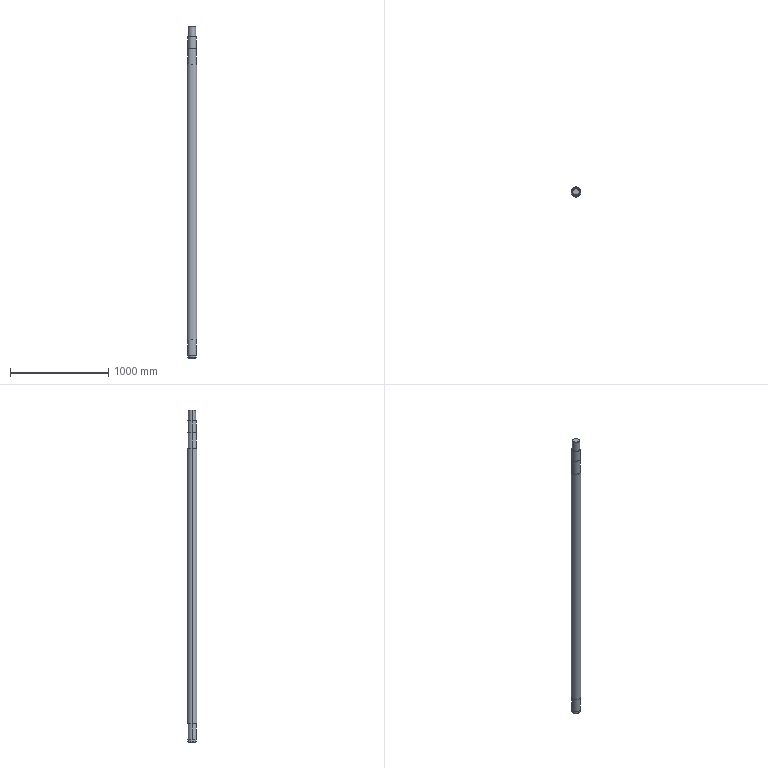Part | SolidWorks | features ICE 7, Chamfer 1, Extrusion 1 | 1 solid | 23 faces | box 100 x 100 x 3375 mm | volume 25329647 mm3 | cylinder 12 | plane 7 | cone 4 | commonest cylinder face diameters 85 x4 90 x4 75 x2 100 x2
STEP:
#1=CARTESIAN_POINT('',(32.5,0.,3610.));
#2=VERTEX_POINT('',#1);
#3=CARTESIAN_POINT('',(-32.5,0.,3610.));
#4=VERTEX_POINT('',#3);
#5=CARTESIAN_POINT('',(0.,0.,3610.));
#6=DIRECTION('',(0.,0.,1.));
#7=DIRECTION('',(1.,0.,0.));
#8=AXIS2_PLACEMENT_3D('',#5,#6,#7);
#9=CIRCLE('',#8,32.5);
#10=EDGE_CURVE('',#2,#4,#9,.T.);
#11=ORIENTED_EDGE('',*,*,#10,.F.);
#12=CARTESIAN_POINT('',(37.5,0.,3605.));
#13=VERTEX_POINT('',#12);
#14=CARTESIAN_POINT('',(32.5,0.,3610.));
#15=DIRECTION('',(0.7071,0.,-0.7071));
#16=VECTOR('',#15,1000.);
#17=LINE('',#14,#16);
#18=EDGE_CURVE('',#2,#13,#17,.T.);
#19=ORIENTED_EDGE('',*,*,#18,.T.);
#20=CARTESIAN_POINT('',(-37.5,0.,3605.));
#21=VERTEX_POINT('',#20);
#22=CARTESIAN_POINT('',(0.,0.,3605.));
#23=DIRECTION('',(0.,0.,-1.));
#24=DIRECTION('',(1.,0.,0.));
#25=AXIS2_PLACEMENT_3D('',#22,#23,#24);
#26=CIRCLE('',#25,37.5);
#27=EDGE_CURVE('',#21,#13,#26,.T.);
#28=ORIENTED_EDGE('',*,*,#27,.F.);
#29=CARTESIAN_POINT('',(-32.5,0.,3610.));
#30=DIRECTION('',(-0.7071,0.,-0.7071));
#31=VECTOR('',#30,1000.);
#32=LINE('',#29,#31);
#33=EDGE_CURVE('',#4,#21,#32,.T.);
#34=ORIENTED_EDGE('',*,*,#33,.F.);
#35=EDGE_LOOP('',(#11,#19,#28,#34));
#36=FACE_OUTER_BOUND('',#35,.T.);
#37=CARTESIAN_POINT('',(0.,0.,3610.));
#38=DIRECTION('',(0.,0.,-1.));
#39=DIRECTION('',(-1.,0.,0.));
#40=AXIS2_PLACEMENT_3D('',#37,#38,#39);
#41=CONICAL_SURFACE('',#40,32.5,0.7854);
#42=ADVANCED_FACE('',(#36),#41,.T.);
#43=CARTESIAN_POINT('',(-37.5,0.,235.));
#44=VERTEX_POINT('',#43);
#45=CARTESIAN_POINT('',(37.5,0.,235.));
#46=VERTEX_POINT('',#45);
#47=CARTESIAN_POINT('',(0.,0.,235.));
#48=DIRECTION('',(0.,0.,-1.));
#49=DIRECTION('',(-1.,0.,0.));
#50=AXIS2_PLACEMENT_3D('',#47,#48,#49);
#51=CIRCLE('',#50,37.5);
#52=EDGE_CURVE('',#44,#46,#51,.T.);
#53=ORIENTED_EDGE('',*,*,#52,.F.);
#54=CARTESIAN_POINT('',(-42.5,0.,240.));
#55=VERTEX_POINT('',#54);
#56=CARTESIAN_POINT('',(-37.5,0.,235.));
#57=DIRECTION('',(-0.7071,0.,0.7071));
#58=VECTOR('',#57,1000.);
#59=LINE('',#56,#58);
#60=EDGE_CURVE('',#44,#55,#59,.T.);
#61=ORIENTED_EDGE('',*,*,#60,.T.);
#62=CARTESIAN_POINT('',(42.5,0.,240.));
#63=VERTEX_POINT('',#62);
#64=CARTESIAN_POINT('',(0.,0.,240.));
#65=DIRECTION('',(0.,0.,1.));
#66=DIRECTION('',(-1.,0.,0.));
#67=AXIS2_PLACEMENT_3D('',#64,#65,#66);
#68=CIRCLE('',#67,42.5);
#69=EDGE_CURVE('',#63,#55,#68,.T.);
#70=ORIENTED_EDGE('',*,*,#69,.F.);
#71=CARTESIAN_POINT('',(37.5,0.,235.));
#72=DIRECTION('',(0.7071,0.,0.7071));
#73=VECTOR('',#72,1000.);
#74=LINE('',#71,#73);
#75=EDGE_CURVE('',#46,#63,#74,.T.);
#76=ORIENTED_EDGE('',*,*,#75,.F.);
#77=EDGE_LOOP('',(#53,#61,#70,#76));
#78=FACE_OUTER_BOUND('',#77,.T.);
#79=CARTESIAN_POINT('',(0.,0.,235.));
#80=DIRECTION('',(0.,0.,1.));
#81=DIRECTION('',(1.,0.,0.));
#82=AXIS2_PLACEMENT_3D('',#79,#80,#81);
#83=CONICAL_SURFACE('',#82,37.5,0.7854);
#84=ADVANCED_FACE('',(#78),#83,.T.);
#85=ORIENTED_EDGE('',*,*,#27,.T.);
#86=CARTESIAN_POINT('',(37.5,0.,3500.));
#87=VERTEX_POINT('',#86);
#88=CARTESIAN_POINT('',(37.5,0.,3610.));
#89=DIRECTION('',(0.,0.,-1.));
#90=VECTOR('',#89,1000.);
#91=LINE('',#88,#90);
#92=EDGE_CURVE('',#13,#87,#91,.T.);
#93=ORIENTED_EDGE('',*,*,#92,.T.);
#94=CARTESIAN_POINT('',(-37.5,0.,3500.));
#95=VERTEX_POINT('',#94);
#96=CARTESIAN_POINT('',(0.,0.,3500.));
#97=DIRECTION('',(0.,0.,1.));
#98=DIRECTION('',(1.,0.,0.));
#99=AXIS2_PLACEMENT_3D('',#96,#97,#98);
#100=CIRCLE('',#99,37.5);
#101=EDGE_CURVE('',#87,#95,#100,.T.);
#102=ORIENTED_EDGE('',*,*,#101,.T.);
#103=CARTESIAN_POINT('',(-37.5,0.,3610.));
#104=DIRECTION('',(0.,0.,-1.));
#105=VECTOR('',#104,1000.);
#106=LINE('',#103,#105);
#107=EDGE_CURVE('',#21,#95,#106,.T.);
#108=ORIENTED_EDGE('',*,*,#107,.F.);
#109=EDGE_LOOP('',(#85,#93,#102,#108));
#110=FACE_OUTER_BOUND('',#109,.T.);
#111=CARTESIAN_POINT('',(0.,0.,3610.));
#112=DIRECTION('',(0.,0.,-1.));
#113=DIRECTION('',(-1.,0.,0.));
#114=AXIS2_PLACEMENT_3D('',#111,#112,#113);
#115=CYLINDRICAL_SURFACE('',#114,37.5);
#116=ADVANCED_FACE('',(#110),#115,.T.);
#117=CARTESIAN_POINT('',(42.5,0.,3500.));
#118=VERTEX_POINT('',#117);
#119=CARTESIAN_POINT('',(-42.5,0.,3500.));
#120=VERTEX_POINT('',#119);
#121=CARTESIAN_POINT('',(0.,0.,3500.));
#122=DIRECTION('',(0.,0.,1.));
#123=DIRECTION('',(1.,0.,0.));
#124=AXIS2_PLACEMENT_3D('',#121,#122,#123);
#125=CIRCLE('',#124,42.5);
#126=EDGE_CURVE('',#118,#120,#125,.T.);
#127=ORIENTED_EDGE('',*,*,#126,.F.);
#128=CARTESIAN_POINT('',(42.5,0.,3380.));
#129=VERTEX_POINT('',#128);
#130=CARTESIAN_POINT('',(42.5,0.,3500.));
#131=DIRECTION('',(0.,0.,-1.));
#132=VECTOR('',#131,1000.);
#133=LINE('',#130,#132);
#134=EDGE_CURVE('',#118,#129,#133,.T.);
#135=ORIENTED_EDGE('',*,*,#134,.T.);
#136=CARTESIAN_POINT('',(-42.5,0.,3380.));
#137=VERTEX_POINT('',#136);
#138=CARTESIAN_POINT('',(0.,0.,3380.));
#139=DIRECTION('',(0.,0.,1.));
#140=DIRECTION('',(1.,0.,0.));
#141=AXIS2_PLACEMENT_3D('',#138,#139,#140);
#142=CIRCLE('',#141,42.5);
#143=EDGE_CURVE('',#129,#137,#142,.T.);
#144=ORIENTED_EDGE('',*,*,#143,.T.);
#145=CARTESIAN_POINT('',(-42.5,0.,3500.));
#146=DIRECTION('',(0.,0.,-1.));
#147=VECTOR('',#146,1000.);
#148=LINE('',#145,#147);
#149=EDGE_CURVE('',#120,#137,#148,.T.);
#150=ORIENTED_EDGE('',*,*,#149,.F.);
#151=EDGE_LOOP('',(#127,#135,#144,#150));
#152=FACE_OUTER_BOUND('',#151,.T.);
#153=CARTESIAN_POINT('',(0.,0.,3500.));
#154=DIRECTION('',(0.,0.,-1.));
#155=DIRECTION('',(-1.,0.,0.));
#156=AXIS2_PLACEMENT_3D('',#153,#154,#155);
#157=CYLINDRICAL_SURFACE('',#156,42.5);
#158=ADVANCED_FACE('',(#152),#157,.T.);
#159=CARTESIAN_POINT('',(45.,0.,3380.));
#160=VERTEX_POINT('',#159);
#161=CARTESIAN_POINT('',(-45.,0.,3380.));
#162=VERTEX_POINT('',#161);
#163=CARTESIAN_POINT('',(0.,0.,3380.));
#164=DIRECTION('',(0.,0.,1.));
#165=DIRECTION('',(1.,0.,0.));
#166=AXIS2_PLACEMENT_3D('',#163,#164,#165);
#167=CIRCLE('',#166,45.);
#168=EDGE_CURVE('',#160,#162,#167,.T.);
#169=ORIENTED_EDGE('',*,*,#168,.F.);
#170=CARTESIAN_POINT('',(45.,0.,3220.));
#171=VERTEX_POINT('',#170);
#172=CARTESIAN_POINT('',(45.,0.,3380.));
#173=DIRECTION('',(0.,0.,-1.));
#174=VECTOR('',#173,1000.);
#175=LINE('',#172,#174);
#176=EDGE_CURVE('',#160,#171,#175,.T.);
#177=ORIENTED_EDGE('',*,*,#176,.T.);
#178=CARTESIAN_POINT('',(-45.,0.,3220.));
#179=VERTEX_POINT('',#178);
#180=CARTESIAN_POINT('',(0.,0.,3220.));
#181=DIRECTION('',(0.,0.,1.));
#182=DIRECTION('',(1.,0.,0.));
#183=AXIS2_PLACEMENT_3D('',#180,#181,#182);
#184=CIRCLE('',#183,45.);
#185=EDGE_CURVE('',#171,#179,#184,.T.);
#186=ORIENTED_EDGE('',*,*,#185,.T.);
#187=CARTESIAN_POINT('',(-45.,0.,3380.));
#188=DIRECTION('',(0.,0.,-1.));
#189=VECTOR('',#188,1000.);
#190=LINE('',#187,#189);
#191=EDGE_CURVE('',#162,#179,#190,.T.);
#192=ORIENTED_EDGE('',*,*,#191,.F.);
#193=EDGE_LOOP('',(#169,#177,#186,#192));
#194=FACE_OUTER_BOUND('',#193,.T.);
#195=CARTESIAN_POINT('',(0.,0.,3380.));
#196=DIRECTION('',(0.,0.,-1.));
#197=DIRECTION('',(-1.,0.,0.));
#198=AXIS2_PLACEMENT_3D('',#195,#196,#197);
#199=CYLINDRICAL_SURFACE('',#198,45.);
#200=ADVANCED_FACE('',(#194),#199,.T.);
#201=CARTESIAN_POINT('',(50.,0.,3220.));
#202=VERTEX_POINT('',#201);
#203=CARTESIAN_POINT('',(-50.,0.,3220.));
#204=VERTEX_POINT('',#203);
#205=CARTESIAN_POINT('',(0.,0.,3220.));
#206=DIRECTION('',(0.,0.,1.));
#207=DIRECTION('',(1.,0.,0.));
#208=AXIS2_PLACEMENT_3D('',#205,#206,#207);
#209=CIRCLE('',#208,50.);
#210=EDGE_CURVE('',#202,#204,#209,.T.);
#211=ORIENTED_EDGE('',*,*,#210,.F.);
#212=CARTESIAN_POINT('',(50.,0.,420.));
#213=VERTEX_POINT('',#212);
#214=CARTESIAN_POINT('',(50.,0.,3220.));
#215=DIRECTION('',(0.,0.,-1.));
#216=VECTOR('',#215,1000.);
#217=LINE('',#214,#216);
#218=EDGE_CURVE('',#202,#213,#217,.T.);
#219=ORIENTED_EDGE('',*,*,#218,.T.);
#220=CARTESIAN_POINT('',(-50.,0.,420.));
#221=VERTEX_POINT('',#220);
#222=CARTESIAN_POINT('',(0.,0.,420.));
#223=DIRECTION('',(0.,0.,1.));
#224=DIRECTION('',(1.,0.,0.));
#225=AXIS2_PLACEMENT_3D('',#222,#223,#224);
#226=CIRCLE('',#225,50.);
#227=EDGE_CURVE('',#213,#221,#226,.T.);
#228=ORIENTED_EDGE('',*,*,#227,.T.);
#229=CARTESIAN_POINT('',(-50.,0.,3220.));
#230=DIRECTION('',(0.,0.,-1.));
#231=VECTOR('',#230,1000.);
#232=LINE('',#229,#231);
#233=EDGE_CURVE('',#204,#221,#232,.T.);
#234=ORIENTED_EDGE('',*,*,#233,.F.);
#235=EDGE_LOOP('',(#211,#219,#228,#234));
#236=FACE_OUTER_BOUND('',#235,.T.);
#237=CARTESIAN_POINT('',(0.,0.,3220.));
#238=DIRECTION('',(0.,0.,-1.));
#239=DIRECTION('',(-1.,0.,0.));
#240=AXIS2_PLACEMENT_3D('',#237,#238,#239);
#241=CYLINDRICAL_SURFACE('',#240,50.);
#242=ADVANCED_FACE('',(#236),#241,.T.);
#243=CARTESIAN_POINT('',(45.,0.,420.));
#244=VERTEX_POINT('',#243);
#245=CARTESIAN_POINT('',(-45.,0.,420.));
#246=VERTEX_POINT('',#245);
#247=CARTESIAN_POINT('',(0.,0.,420.));
#248=DIRECTION('',(0.,0.,1.));
#249=DIRECTION('',(1.,0.,0.));
#250=AXIS2_PLACEMENT_3D('',#247,#248,#249);
#251=CIRCLE('',#250,45.);
#252=EDGE_CURVE('',#244,#246,#251,.T.);
#253=ORIENTED_EDGE('',*,*,#252,.F.);
#254=CARTESIAN_POINT('',(45.,0.,260.));
#255=VERTEX_POINT('',#254);
#256=CARTESIAN_POINT('',(45.,0.,420.));
#257=DIRECTION('',(0.,0.,-1.));
#258=VECTOR('',#257,1000.);
#259=LINE('',#256,#258);
#260=EDGE_CURVE('',#244,#255,#259,.T.);
#261=ORIENTED_EDGE('',*,*,#260,.T.);
#262=CARTESIAN_POINT('',(-45.,0.,260.));
#263=VERTEX_POINT('',#262);
#264=CARTESIAN_POINT('',(0.,0.,260.));
#265=DIRECTION('',(0.,0.,1.));
#266=DIRECTION('',(1.,0.,0.));
#267=AXIS2_PLACEMENT_3D('',#264,#265,#266);
#268=CIRCLE('',#267,45.);
#269=EDGE_CURVE('',#255,#263,#268,.T.);
#270=ORIENTED_EDGE('',*,*,#269,.T.);
#271=CARTESIAN_POINT('',(-45.,0.,420.));
#272=DIRECTION('',(0.,0.,-1.));
#273=VECTOR('',#272,1000.);
#274=LINE('',#271,#273);
#275=EDGE_CURVE('',#246,#263,#274,.T.);
#276=ORIENTED_EDGE('',*,*,#275,.F.);
#277=EDGE_LOOP('',(#253,#261,#270,#276));
#278=FACE_OUTER_BOUND('',#277,.T.);
#279=CARTESIAN_POINT('',(0.,0.,420.));
#280=DIRECTION('',(0.,0.,-1.));
#281=DIRECTION('',(-1.,0.,0.));
#282=AXIS2_PLACEMENT_3D('',#279,#280,#281);
#283=CYLINDRICAL_SURFACE('',#282,45.);
#284=ADVANCED_FACE('',(#278),#283,.T.);
#285=CARTESIAN_POINT('',(42.5,0.,260.));
#286=VERTEX_POINT('',#285);
#287=CARTESIAN_POINT('',(-42.5,0.,260.));
#288=VERTEX_POINT('',#287);
#289=CARTESIAN_POINT('',(0.,0.,260.));
#290=DIRECTION('',(0.,0.,1.));
#291=DIRECTION('',(1.,0.,0.));
#292=AXIS2_PLACEMENT_3D('',#289,#290,#291);
#293=CIRCLE('',#292,42.5);
#294=EDGE_CURVE('',#286,#288,#293,.T.);
#295=ORIENTED_EDGE('',*,*,#294,.F.);
#296=CARTESIAN_POINT('',(42.5,0.,260.));
#297=DIRECTION('',(0.,0.,-1.));
#298=VECTOR('',#297,1000.);
#299=LINE('',#296,#298);
#300=EDGE_CURVE('',#286,#63,#299,.T.);
#301=ORIENTED_EDGE('',*,*,#300,.T.);
#302=ORIENTED_EDGE('',*,*,#69,.T.);
#303=CARTESIAN_POINT('',(-42.5,0.,260.));
#304=DIRECTION('',(0.,0.,-1.));
#305=VECTOR('',#304,1000.);
#306=LINE('',#303,#305);
#307=EDGE_CURVE('',#288,#55,#306,.T.);
#308=ORIENTED_EDGE('',*,*,#307,.F.);
#309=EDGE_LOOP('',(#295,#301,#302,#308));
#310=FACE_OUTER_BOUND('',#309,.T.);
#311=CARTESIAN_POINT('',(0.,0.,260.));
#312=DIRECTION('',(0.,0.,-1.));
#313=DIRECTION('',(-1.,0.,0.));
#314=AXIS2_PLACEMENT_3D('',#311,#312,#313);
#315=CYLINDRICAL_SURFACE('',#314,42.5);
#316=ADVANCED_FACE('',(#310),#315,.T.);
#317=ORIENTED_EDGE('',*,*,#300,.F.);
#318=CARTESIAN_POINT('',(0.,0.,260.));
#319=DIRECTION('',(0.,0.,1.));
#320=DIRECTION('',(1.,0.,0.));
#321=AXIS2_PLACEMENT_3D('',#318,#319,#320);
#322=CIRCLE('',#321,42.5);
#323=EDGE_CURVE('',#288,#286,#322,.T.);
#324=ORIENTED_EDGE('',*,*,#323,.F.);
#325=ORIENTED_EDGE('',*,*,#307,.T.);
#326=CARTESIAN_POINT('',(0.,0.,240.));
#327=DIRECTION('',(0.,0.,1.));
#328=DIRECTION('',(-1.,0.,0.));
#329=AXIS2_PLACEMENT_3D('',#326,#327,#328);
#330=CIRCLE('',#329,42.5);
#331=EDGE_CURVE('',#55,#63,#330,.T.);
#332=ORIENTED_EDGE('',*,*,#331,.T.);
#333=EDGE_LOOP('',(#317,#324,#325,#332));
#334=FACE_OUTER_BOUND('',#333,.T.);
#335=CARTESIAN_POINT('',(0.,0.,260.));
#336=DIRECTION('',(0.,0.,-1.));
#337=DIRECTION('',(-1.,0.,0.));
#338=AXIS2_PLACEMENT_3D('',#335,#336,#337);
#339=CYLINDRICAL_SURFACE('',#338,42.5);
#340=ADVANCED_FACE('',(#334),#339,.T.);
#341=ORIENTED_EDGE('',*,*,#260,.F.);
#342=CARTESIAN_POINT('',(0.,0.,420.));
#343=DIRECTION('',(0.,0.,1.));
#344=DIRECTION('',(1.,0.,0.));
#345=AXIS2_PLACEMENT_3D('',#342,#343,#344);
#346=CIRCLE('',#345,45.);
#347=EDGE_CURVE('',#246,#244,#346,.T.);
#348=ORIENTED_EDGE('',*,*,#347,.F.);
#349=ORIENTED_EDGE('',*,*,#275,.T.);
#350=CARTESIAN_POINT('',(0.,0.,260.));
#351=DIRECTION('',(0.,0.,1.));
#352=DIRECTION('',(1.,0.,0.));
#353=AXIS2_PLACEMENT_3D('',#350,#351,#352);
#354=CIRCLE('',#353,45.);
#355=EDGE_CURVE('',#263,#255,#354,.T.);
#356=ORIENTED_EDGE('',*,*,#355,.T.);
#357=EDGE_LOOP('',(#341,#348,#349,#356));
#358=FACE_OUTER_BOUND('',#357,.T.);
#359=CARTESIAN_POINT('',(0.,0.,420.));
#360=DIRECTION('',(0.,0.,-1.));
#361=DIRECTION('',(-1.,0.,0.));
#362=AXIS2_PLACEMENT_3D('',#359,#360,#361);
#363=CYLINDRICAL_SURFACE('',#362,45.);
#364=ADVANCED_FACE('',(#358),#363,.T.);
#365=ORIENTED_EDGE('',*,*,#323,.T.);
#366=ORIENTED_EDGE('',*,*,#294,.T.);
#367=EDGE_LOOP('',(#365,#366));
#368=FACE_BOUND('',#367,.T.);
#369=ORIENTED_EDGE('',*,*,#355,.F.);
#370=ORIENTED_EDGE('',*,*,#269,.F.);
#371=EDGE_LOOP('',(#369,#370));
#372=FACE_OUTER_BOUND('',#371,.T.);
#373=CARTESIAN_POINT('',(0.,0.,260.));
#374=DIRECTION('',(0.,0.,1.));
#375=DIRECTION('',(1.,0.,0.));
#376=AXIS2_PLACEMENT_3D('',#373,#374,#375);
#377=PLANE('',#376);
#378=ADVANCED_FACE('',(#368,#372),#377,.F.);
#379=ORIENTED_EDGE('',*,*,#218,.F.);
#380=CARTESIAN_POINT('',(0.,0.,3220.));
#381=DIRECTION('',(0.,0.,1.));
#382=DIRECTION('',(1.,0.,0.));
#383=AXIS2_PLACEMENT_3D('',#380,#381,#382);
#384=CIRCLE('',#383,50.);
#385=EDGE_CURVE('',#204,#202,#384,.T.);
#386=ORIENTED_EDGE('',*,*,#385,.F.);
#387=ORIENTED_EDGE('',*,*,#233,.T.);
#388=CARTESIAN_POINT('',(0.,0.,420.));
#389=DIRECTION('',(0.,0.,1.));
#390=DIRECTION('',(1.,0.,0.));
#391=AXIS2_PLACEMENT_3D('',#388,#389,#390);
#392=CIRCLE('',#391,50.);
#393=EDGE_CURVE('',#221,#213,#392,.T.);
#394=ORIENTED_EDGE('',*,*,#393,.T.);
#395=EDGE_LOOP('',(#379,#386,#387,#394));
#396=FACE_OUTER_BOUND('',#395,.T.);
#397=CARTESIAN_POINT('',(0.,0.,3220.));
#398=DIRECTION('',(0.,0.,-1.));
#399=DIRECTION('',(-1.,0.,0.));
#400=AXIS2_PLACEMENT_3D('',#397,#398,#399);
#401=CYLINDRICAL_SURFACE('',#400,50.);
#402=ADVANCED_FACE('',(#396),#401,.T.);
#403=CARTESIAN_POINT('',(0.,0.,3220.));
#404=DIRECTION('',(0.,0.,1.));
#405=DIRECTION('',(1.,0.,0.));
#406=AXIS2_PLACEMENT_3D('',#403,#404,#405);
#407=CIRCLE('',#406,45.);
#408=EDGE_CURVE('',#179,#171,#407,.T.);
#409=ORIENTED_EDGE('',*,*,#408,.F.);
#410=ORIENTED_EDGE('',*,*,#185,.F.);
#411=EDGE_LOOP('',(#409,#410));
#412=FACE_BOUND('',#411,.T.);
#413=ORIENTED_EDGE('',*,*,#385,.T.);
#414=ORIENTED_EDGE('',*,*,#210,.T.);
#415=EDGE_LOOP('',(#413,#414));
#416=FACE_OUTER_BOUND('',#415,.T.);
#417=CARTESIAN_POINT('',(0.,0.,3220.));
#418=DIRECTION('',(0.,0.,1.));
#419=DIRECTION('',(1.,0.,0.));
#420=AXIS2_PLACEMENT_3D('',#417,#418,#419);
#421=PLANE('',#420);
#422=ADVANCED_FACE('',(#412,#416),#421,.T.);
#423=ORIENTED_EDGE('',*,*,#347,.T.);
#424=ORIENTED_EDGE('',*,*,#252,.T.);
#425=EDGE_LOOP('',(#423,#424));
#426=FACE_BOUND('',#425,.T.);
#427=ORIENTED_EDGE('',*,*,#393,.F.);
#428=ORIENTED_EDGE('',*,*,#227,.F.);
#429=EDGE_LOOP('',(#427,#428));
#430=FACE_OUTER_BOUND('',#429,.T.);
#431=CARTESIAN_POINT('',(0.,0.,420.));
#432=DIRECTION('',(0.,0.,1.));
#433=DIRECTION('',(1.,0.,0.));
#434=AXIS2_PLACEMENT_3D('',#431,#432,#433);
#435=PLANE('',#434);
#436=ADVANCED_FACE('',(#426,#430),#435,.F.);
#437=ORIENTED_EDGE('',*,*,#176,.F.);
#438=CARTESIAN_POINT('',(0.,0.,3380.));
#439=DIRECTION('',(0.,0.,1.));
#440=DIRECTION('',(1.,0.,0.));
#441=AXIS2_PLACEMENT_3D('',#438,#439,#440);
#442=CIRCLE('',#441,45.);
#443=EDGE_CURVE('',#162,#160,#442,.T.);
#444=ORIENTED_EDGE('',*,*,#443,.F.);
#445=ORIENTED_EDGE('',*,*,#191,.T.);
#446=ORIENTED_EDGE('',*,*,#408,.T.);
#447=EDGE_LOOP('',(#437,#444,#445,#446));
#448=FACE_OUTER_BOUND('',#447,.T.);
#449=CARTESIAN_POINT('',(0.,0.,3380.));
#450=DIRECTION('',(0.,0.,-1.));
#451=DIRECTION('',(-1.,0.,0.));
#452=AXIS2_PLACEMENT_3D('',#449,#450,#451);
#453=CYLINDRICAL_SURFACE('',#452,45.);
#454=ADVANCED_FACE('',(#448),#453,.T.);
#455=CARTESIAN_POINT('',(0.,0.,3380.));
#456=DIRECTION('',(0.,0.,1.));
#457=DIRECTION('',(1.,0.,0.));
#458=AXIS2_PLACEMENT_3D('',#455,#456,#457);
#459=CIRCLE('',#458,42.5);
#460=EDGE_CURVE('',#137,#129,#459,.T.);
#461=ORIENTED_EDGE('',*,*,#460,.F.);
#462=ORIENTED_EDGE('',*,*,#143,.F.);
#463=EDGE_LOOP('',(#461,#462));
#464=FACE_BOUND('',#463,.T.);
#465=ORIENTED_EDGE('',*,*,#443,.T.);
#466=ORIENTED_EDGE('',*,*,#168,.T.);
#467=EDGE_LOOP('',(#465,#466));
#468=FACE_OUTER_BOUND('',#467,.T.);
#469=CARTESIAN_POINT('',(0.,0.,3380.));
#470=DIRECTION('',(0.,0.,1.));
#471=DIRECTION('',(1.,0.,0.));
#472=AXIS2_PLACEMENT_3D('',#469,#470,#471);
#473=PLANE('',#472);
#474=ADVANCED_FACE('',(#464,#468),#473,.T.);
#475=ORIENTED_EDGE('',*,*,#134,.F.);
#476=CARTESIAN_POINT('',(0.,0.,3500.));
#477=DIRECTION('',(0.,0.,1.));
#478=DIRECTION('',(1.,0.,0.));
#479=AXIS2_PLACEMENT_3D('',#476,#477,#478);
#480=CIRCLE('',#479,42.5);
#481=EDGE_CURVE('',#120,#118,#480,.T.);
#482=ORIENTED_EDGE('',*,*,#481,.F.);
#483=ORIENTED_EDGE('',*,*,#149,.T.);
#484=ORIENTED_EDGE('',*,*,#460,.T.);
#485=EDGE_LOOP('',(#475,#482,#483,#484));
#486=FACE_OUTER_BOUND('',#485,.T.);
#487=CARTESIAN_POINT('',(0.,0.,3500.));
#488=DIRECTION('',(0.,0.,-1.));
#489=DIRECTION('',(-1.,0.,0.));
#490=AXIS2_PLACEMENT_3D('',#487,#488,#489);
#491=CYLINDRICAL_SURFACE('',#490,42.5);
#492=ADVANCED_FACE('',(#486),#491,.T.);
#493=CARTESIAN_POINT('',(0.,0.,3500.));
#494=DIRECTION('',(0.,0.,1.));
#495=DIRECTION('',(1.,0.,0.));
#496=AXIS2_PLACEMENT_3D('',#493,#494,#495);
#497=CIRCLE('',#496,37.5);
#498=EDGE_CURVE('',#95,#87,#497,.T.);
#499=ORIENTED_EDGE('',*,*,#498,.F.);
#500=ORIENTED_EDGE('',*,*,#101,.F.);
#501=EDGE_LOOP('',(#499,#500));
#502=FACE_BOUND('',#501,.T.);
#503=ORIENTED_EDGE('',*,*,#481,.T.);
#504=ORIENTED_EDGE('',*,*,#126,.T.);
#505=EDGE_LOOP('',(#503,#504));
#506=FACE_OUTER_BOUND('',#505,.T.);
#507=CARTESIAN_POINT('',(0.,0.,3500.));
#508=DIRECTION('',(0.,0.,1.));
#509=DIRECTION('',(1.,0.,0.));
#510=AXIS2_PLACEMENT_3D('',#507,#508,#509);
#511=PLANE('',#510);
#512=ADVANCED_FACE('',(#502,#506),#511,.T.);
#513=ORIENTED_EDGE('',*,*,#92,.F.);
#514=CARTESIAN_POINT('',(0.,0.,3605.));
#515=DIRECTION('',(0.,0.,-1.));
#516=DIRECTION('',(1.,0.,0.));
#517=AXIS2_PLACEMENT_3D('',#514,#515,#516);
#518=CIRCLE('',#517,37.5);
#519=EDGE_CURVE('',#13,#21,#518,.T.);
#520=ORIENTED_EDGE('',*,*,#519,.T.);
#521=ORIENTED_EDGE('',*,*,#107,.T.);
#522=ORIENTED_EDGE('',*,*,#498,.T.);
#523=EDGE_LOOP('',(#513,#520,#521,#522));
#524=FACE_OUTER_BOUND('',#523,.T.);
#525=CARTESIAN_POINT('',(0.,0.,3610.));
#526=DIRECTION('',(0.,0.,-1.));
#527=DIRECTION('',(-1.,0.,0.));
#528=AXIS2_PLACEMENT_3D('',#525,#526,#527);
#529=CYLINDRICAL_SURFACE('',#528,37.5);
#530=ADVANCED_FACE('',(#524),#529,.T.);
#531=CARTESIAN_POINT('',(0.,0.,3610.));
#532=DIRECTION('',(0.,0.,1.));
#533=DIRECTION('',(1.,0.,0.));
#534=AXIS2_PLACEMENT_3D('',#531,#532,#533);
#535=CIRCLE('',#534,32.5);
#536=EDGE_CURVE('',#4,#2,#535,.T.);
#537=ORIENTED_EDGE('',*,*,#536,.T.);
#538=ORIENTED_EDGE('',*,*,#10,.T.);
#539=EDGE_LOOP('',(#537,#538));
#540=FACE_OUTER_BOUND('',#539,.T.);
#541=CARTESIAN_POINT('',(0.,0.,3610.));
#542=DIRECTION('',(0.,0.,1.));
#543=DIRECTION('',(1.,0.,0.));
#544=AXIS2_PLACEMENT_3D('',#541,#542,#543);
#545=PLANE('',#544);
#546=ADVANCED_FACE('',(#540),#545,.T.);
#547=CARTESIAN_POINT('',(0.,0.,235.));
#548=DIRECTION('',(0.,0.,-1.));
#549=DIRECTION('',(-1.,0.,0.));
#550=AXIS2_PLACEMENT_3D('',#547,#548,#549);
#551=CIRCLE('',#550,37.5);
#552=EDGE_CURVE('',#46,#44,#551,.T.);
#553=ORIENTED_EDGE('',*,*,#552,.T.);
#554=ORIENTED_EDGE('',*,*,#52,.T.);
#555=EDGE_LOOP('',(#553,#554));
#556=FACE_OUTER_BOUND('',#555,.T.);
#557=CARTESIAN_POINT('',(0.,0.,235.));
#558=DIRECTION('',(0.,0.,-1.));
#559=DIRECTION('',(-1.,0.,0.));
#560=AXIS2_PLACEMENT_3D('',#557,#558,#559);
#561=PLANE('',#560);
#562=ADVANCED_FACE('',(#556),#561,.T.);
#563=ORIENTED_EDGE('',*,*,#60,.F.);
#564=ORIENTED_EDGE('',*,*,#552,.F.);
#565=ORIENTED_EDGE('',*,*,#75,.T.);
#566=ORIENTED_EDGE('',*,*,#331,.F.);
#567=EDGE_LOOP('',(#563,#564,#565,#566));
#568=FACE_OUTER_BOUND('',#567,.T.);
#569=CARTESIAN_POINT('',(0.,0.,235.));
#570=DIRECTION('',(0.,0.,1.));
#571=DIRECTION('',(1.,0.,0.));
#572=AXIS2_PLACEMENT_3D('',#569,#570,#571);
#573=CONICAL_SURFACE('',#572,37.5,0.7854);
#574=ADVANCED_FACE('',(#568),#573,.T.);
#575=ORIENTED_EDGE('',*,*,#18,.F.);
#576=ORIENTED_EDGE('',*,*,#536,.F.);
#577=ORIENTED_EDGE('',*,*,#33,.T.);
#578=ORIENTED_EDGE('',*,*,#519,.F.);
#579=EDGE_LOOP('',(#575,#576,#577,#578));
#580=FACE_OUTER_BOUND('',#579,.T.);
#581=CARTESIAN_POINT('',(0.,0.,3610.));
#582=DIRECTION('',(0.,0.,-1.));
#583=DIRECTION('',(-1.,0.,0.));
#584=AXIS2_PLACEMENT_3D('',#581,#582,#583);
#585=CONICAL_SURFACE('',#584,32.5,0.7854);
#586=ADVANCED_FACE('',(#580),#585,.T.);
#587=CLOSED_SHELL('',(#42,#84,#116,#158,#200,#242,#284,#316,#340,#364,#378,#402,#422,#436,#454,#474,#492,#512,#530,#546,#562,#574,#586));
#588=MANIFOLD_SOLID_BREP('',#587);
#589=CARTESIAN_POINT('',(0.,0.,0.));
#590=DIRECTION('',(0.,0.,1.));
#591=DIRECTION('',(1.,0.,0.));
#592=AXIS2_PLACEMENT_3D('',#589,#590,#591);
#593=(LENGTH_UNIT()NAMED_UNIT(*)SI_UNIT(.MILLI.,.METRE.));
#594=UNCERTAINTY_MEASURE_WITH_UNIT(LENGTH_MEASURE(0.00001),#593,'','');
#595=(NAMED_UNIT(*)PLANE_ANGLE_UNIT()SI_UNIT($,.RADIAN.));
#596=(NAMED_UNIT(*)SI_UNIT($,.STERADIAN.)SOLID_ANGLE_UNIT());
#597=(GEOMETRIC_REPRESENTATION_CONTEXT(3)GLOBAL_UNCERTAINTY_ASSIGNED_CONTEXT((#594))GLOBAL_UNIT_ASSIGNED_CONTEXT((#593,#595,#596))REPRESENTATION_CONTEXT('',''));
#598=ADVANCED_BREP_SHAPE_REPRESENTATION('',(#588,#592),#597);